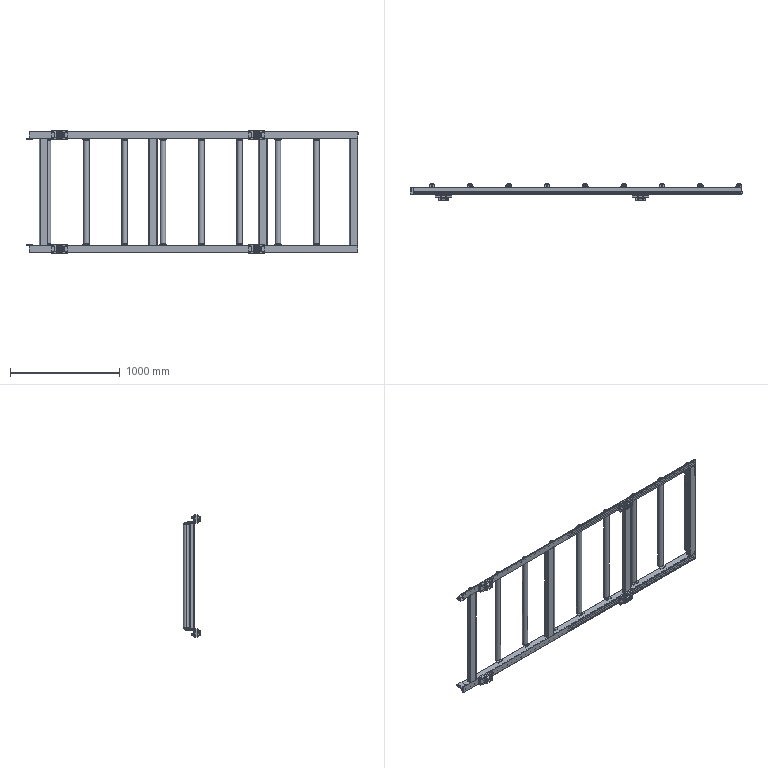Part | SolidWorks | features ReferencePattern 33, LocalLPattern 3 | 61 solids | 4228 faces | volume 28545845 mm3 | plane 2434 | cylinder 998 | spline 640 | cone 108 | torus 40 | sphere 8 | commonest cylinder face diameters 6 x200 9.5 x200 2.258 x96 15 x68 9 x64 16 x52